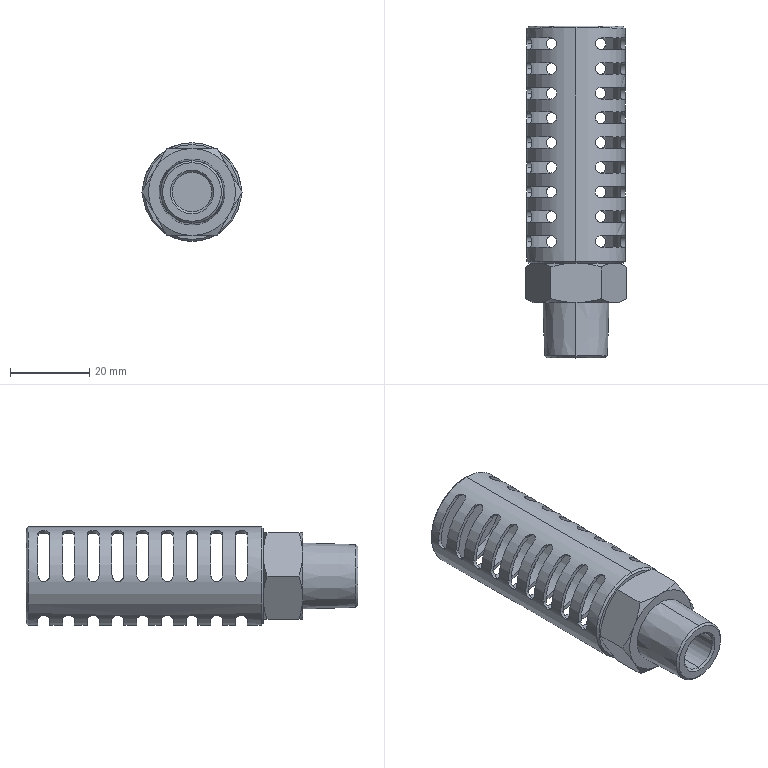Part | STEP file | VBA22A-03GN_AN6009 Silencer | 1 solid | 175 faces | box 25.403 x 84 x 25 mm | volume 9196 mm3 | cylinder 87 | plane 66 | cone 22 | commonest cylinder face diameters 3 x81 10 x2 23 x2 25 x2